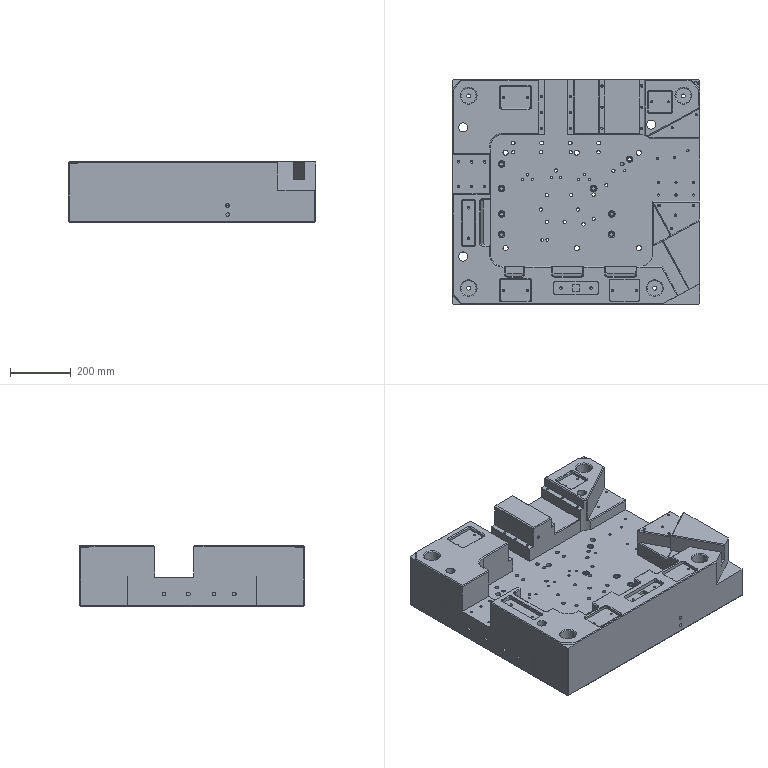Part | Creo | 1 solid | 767 faces | box 815 x 740 x 200 mm | volume 74525593 mm3 | cylinder 368 | plane 273 | cone 118 | spline 8 | commonest cylinder face diameters 11 x50 12 x50 7.2 x42 8 x36 13 x16 17.5 x16